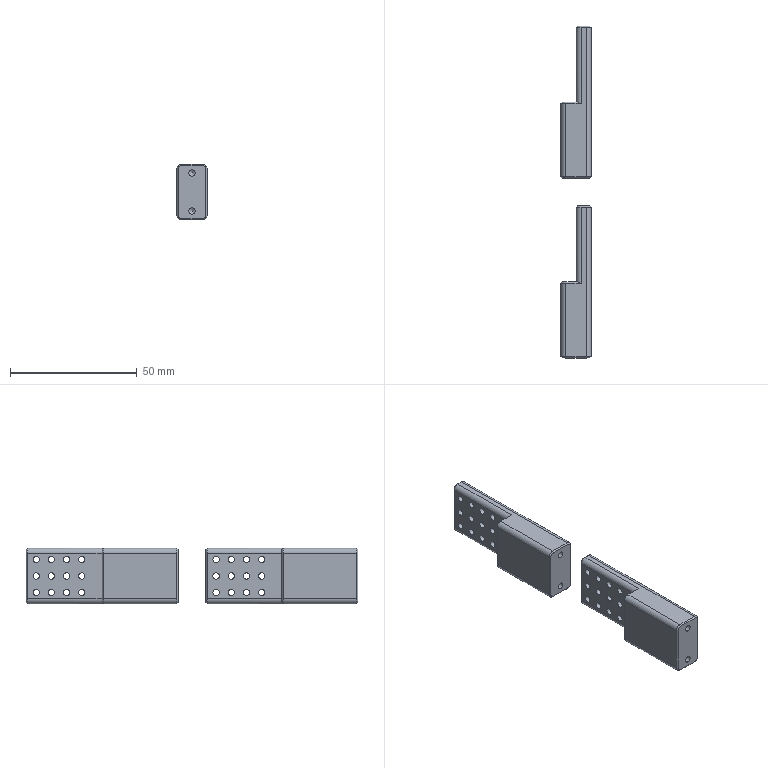CAM job | NX | 3+2 milling, drilling | part box 12 x 131 x 22 mm | stock box 15 x 135 x 25 mm
Tools:
number,name,description,diameter,corner_radius,flute_length,length,flutes
9,D10,平底铣刀-粗,10.0,0.0,35.0,75.0,2
10,D10-J,平底铣刀-精,10.0,0.0,35.0,75.0,2
17,D6R0.5,圆鼻刀-粗,6.0,0.5,50.0,75.0,2
1,D80R0.8飞刀,圆鼻刀-粗,80.0,0.8,50.0,75.0,2
1,D80R0.8飞刀-J,圆鼻刀-精,80.0,0.8,50.0,75.0,2
2,D6倒角刀,倒角刀,6.0,0.0,3.0,25.0,2
20,M3X0.5,丝锥,2.5,0.0,35.0,50.0,2
12,钻头2.5,Twist Drill 2.5 mm,2.5,0.0,30.0,32.0,2
Operations:
program,operation,operation_type,tool,method,geometry_group,spindle_rpm,surface_speed,feed_per_tooth,feed_cut,feed_plunge,cut_length_mm,path_length_mm,cut_time_min,machine_time_min
B,底壁铣飞面一刀开粗_COPY,VolumeBased25DMillingOperation,D80R0.8飞刀,分层开粗-切深K-步距G,W-B,2800.0,703.696,0.5357,3000.0,100.0,1435.164,2714.186,0.4784,0.6063
B,底壁铣飞面一刀精光_COPY,VolumeBased25DMillingOperation,D80R0.8飞刀-J,侧刃精光-切深K-步距G,W-B,4000.0,1005.28,0.125,1000.0,100.0,238.998,274.998,0.239,0.2426
B,型腔铣开粗-中_COPY,CavityMilling,D10,分层开粗-切深K-步距G,W-B,8000.0,251.32,0.25,4000.0,100.0,9402.06,11137.594,2.35,2.623
B,等高精光往复爬面_COPY_COPY,ZLevelMilling,D6R0.5,等高爬面-切深K-步距G,W-B,7000.0,131.947,0.3214,4500.0,100.0,6624.02,6855.097,1.472,1.495
B,钻倒角_2,Operation,D6倒角刀,METHOD,W-B,7000.0,131.947,0.0357,500.0,0.0,114.0,551.468,0.228,0.2717
B,底壁铣倒角_COPY_1,VolumeBased25DMillingOperation,D6倒角刀,爬面_倒角-切深0-步距G,W-B,6500.0,122.519,0.1154,1500.0,100.0,207.577,672.009,0.1384,0.1848
B,底壁铣精光底面-中_COPY,VolumeBased25DMillingOperation,D10-J,精光步距切深关,W-B,7000.0,175.0,0.0536,1500.0,100.0,450.979,576.132,0.3007,0.3132
B,等高精光-中_COPY,ZLevelMilling,D10-J,侧刃精光-切深K-步距G,W-B,8000.0,251.32,0.0625,1000.0,100.0,74.067,203.718,0.0741,0.087
B,等高精光往复爬面_COPY_COPY_COPY,ZLevelMilling,D6R0.5,等高爬面-切深K-步距G,W-B,7000.0,131.947,0.2143,3000.0,100.0,5539.394,5883.442,1.847,1.881
A,顶面,FaceMilling,D80R0.8飞刀,侧刃精光-切深K-步距G,W-A,5000.0,1256.637,0.1,1000.0,100.0,225.0,261.0,0.225,0.2286
A,外形粗_2,VolumeBased25DMillingOperation,D10,METHOD,W-A,8000.0,251.327,0.3125,5000.0,80.0,6628.723,6801.823,1.326,1.343
A,打点-深0.8,Operation,D6倒角刀,NONE,W-A,8000.0,150.796,0.0312,500.0,90.0,43.2,338.205,0.0864,0.1159
A,通孔-M3螺纹底孔,Operation,钻头2.5,NONE,W-A,3000.0,23.562,0.05,300.0,90.0,306.026,863.857,1.02,1.076
A,等高精光往复爬面_COPY,ZLevelMilling,D6R0.5,等高爬面-切深K-步距G,W-A,7000.0,131.947,0.3214,4500.0,100.0,11433.277,11680.049,2.541,2.565
A,钻倒角_1,Operation,D6倒角刀,METHOD,W-A,8000.0,150.796,0.0312,500.0,0.0,114.0,539.468,0.228,0.2705
A,底壁铣倒角_COPY,VolumeBased25DMillingOperation,D6倒角刀,爬面_倒角-切深0-步距G,W-A,6500.0,122.519,0.1154,1500.0,100.0,157.014,407.802,0.1047,0.1298
A,通孔-攻牙M3,Operation,M3X0.5,METHOD,W-A,800.0,6.283,0.0003,0.5,90.0,240.0,731.805,480.0,480.049
A,外形半精_2,VolumeBased25DMillingOperation,D10-J,METHOD,W-A,8000.0,251.327,0.0625,1000.0,100.0,398.488,623.288,0.3985,0.421